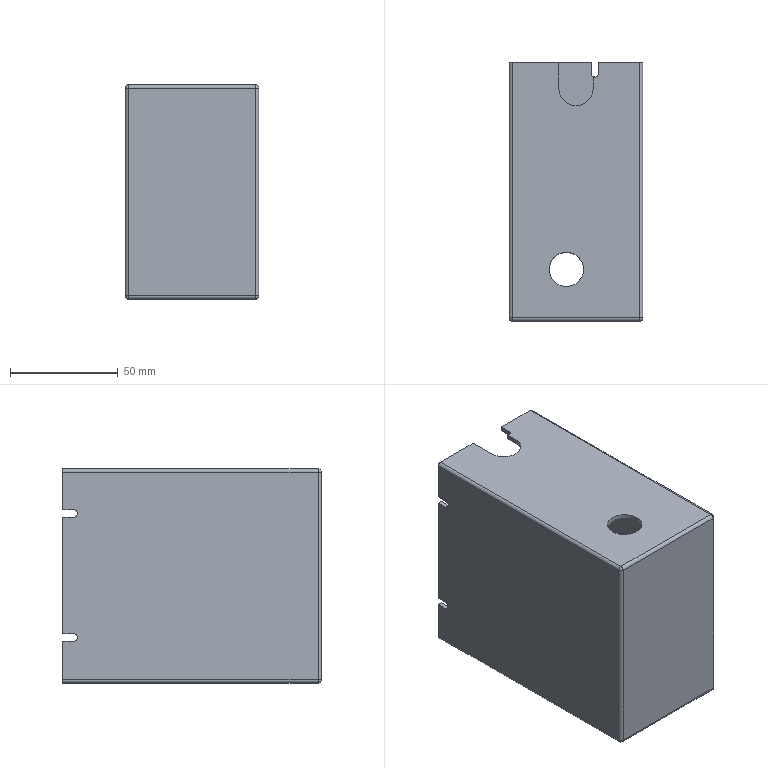Part | STEP file | 1 solid | 52 faces | box 62 x 120 x 99.5 mm | volume 84647 mm3 | plane 29 | cylinder 19 | sphere 4 | commonest cylinder face diameters 3 x8 3.5 x6 16 x5